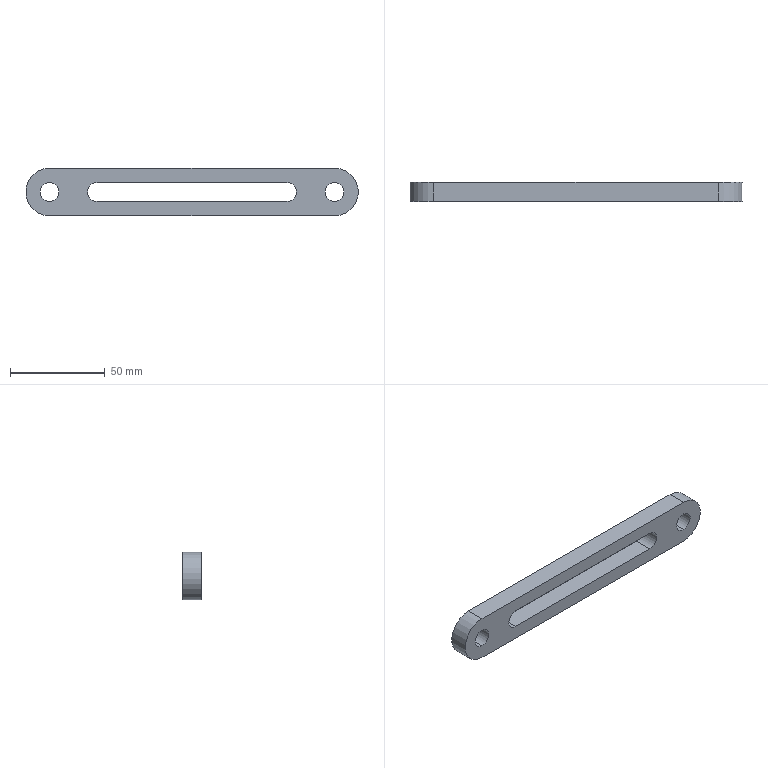Part | SolidWorks | features Extrusion 1, ICE 1 | 1 solid | 14 faces | box 175 x 10 x 25 mm | volume 30053 mm3 | cylinder 8 | plane 6 | commonest cylinder face diameters 10 x6 25 x2
STEP:
#1=CARTESIAN_POINT('',(150.,5.,-5.));
#2=VERTEX_POINT('',#1);
#3=CARTESIAN_POINT('',(150.,5.,5.));
#4=VERTEX_POINT('',#3);
#5=CARTESIAN_POINT('',(150.,5.,0.));
#6=DIRECTION('',(0.,1.,0.));
#7=DIRECTION('',(0.,0.,1.));
#8=AXIS2_PLACEMENT_3D('',#5,#6,#7);
#9=CIRCLE('',#8,5.);
#10=EDGE_CURVE('',#2,#4,#9,.T.);
#11=ORIENTED_EDGE('',*,*,#10,.T.);
#12=CARTESIAN_POINT('',(150.,-5.,5.));
#13=VERTEX_POINT('',#12);
#14=CARTESIAN_POINT('',(150.,5.,5.));
#15=DIRECTION('',(0.,-1.,0.));
#16=VECTOR('',#15,1000.);
#17=LINE('',#14,#16);
#18=EDGE_CURVE('',#4,#13,#17,.T.);
#19=ORIENTED_EDGE('',*,*,#18,.T.);
#20=CARTESIAN_POINT('',(150.,-5.,-5.));
#21=VERTEX_POINT('',#20);
#22=CARTESIAN_POINT('',(150.,-5.,0.));
#23=DIRECTION('',(0.,1.,0.));
#24=DIRECTION('',(0.,0.,1.));
#25=AXIS2_PLACEMENT_3D('',#22,#23,#24);
#26=CIRCLE('',#25,5.);
#27=EDGE_CURVE('',#21,#13,#26,.T.);
#28=ORIENTED_EDGE('',*,*,#27,.F.);
#29=CARTESIAN_POINT('',(150.,5.,-5.));
#30=DIRECTION('',(0.,-1.,0.));
#31=VECTOR('',#30,1000.);
#32=LINE('',#29,#31);
#33=EDGE_CURVE('',#2,#21,#32,.T.);
#34=ORIENTED_EDGE('',*,*,#33,.F.);
#35=EDGE_LOOP('',(#11,#19,#28,#34));
#36=FACE_OUTER_BOUND('',#35,.T.);
#37=CARTESIAN_POINT('',(150.,5.,0.));
#38=DIRECTION('',(0.,-1.,0.));
#39=DIRECTION('',(0.,0.,-1.));
#40=AXIS2_PLACEMENT_3D('',#37,#38,#39);
#41=CYLINDRICAL_SURFACE('',#40,5.);
#42=ADVANCED_FACE('',(#36),#41,.F.);
#43=CARTESIAN_POINT('',(0.,5.,-5.));
#44=VERTEX_POINT('',#43);
#45=CARTESIAN_POINT('',(0.,5.,5.));
#46=VERTEX_POINT('',#45);
#47=CARTESIAN_POINT('',(0.,5.,0.));
#48=DIRECTION('',(0.,1.,0.));
#49=DIRECTION('',(0.,0.,1.));
#50=AXIS2_PLACEMENT_3D('',#47,#48,#49);
#51=CIRCLE('',#50,5.);
#52=EDGE_CURVE('',#44,#46,#51,.T.);
#53=ORIENTED_EDGE('',*,*,#52,.T.);
#54=CARTESIAN_POINT('',(0.,-5.,5.));
#55=VERTEX_POINT('',#54);
#56=CARTESIAN_POINT('',(0.,5.,5.));
#57=DIRECTION('',(0.,-1.,0.));
#58=VECTOR('',#57,1000.);
#59=LINE('',#56,#58);
#60=EDGE_CURVE('',#46,#55,#59,.T.);
#61=ORIENTED_EDGE('',*,*,#60,.T.);
#62=CARTESIAN_POINT('',(0.,-5.,-5.));
#63=VERTEX_POINT('',#62);
#64=CARTESIAN_POINT('',(0.,-5.,0.));
#65=DIRECTION('',(0.,1.,0.));
#66=DIRECTION('',(0.,0.,1.));
#67=AXIS2_PLACEMENT_3D('',#64,#65,#66);
#68=CIRCLE('',#67,5.);
#69=EDGE_CURVE('',#63,#55,#68,.T.);
#70=ORIENTED_EDGE('',*,*,#69,.F.);
#71=CARTESIAN_POINT('',(0.,5.,-5.));
#72=DIRECTION('',(0.,-1.,0.));
#73=VECTOR('',#72,1000.);
#74=LINE('',#71,#73);
#75=EDGE_CURVE('',#44,#63,#74,.T.);
#76=ORIENTED_EDGE('',*,*,#75,.F.);
#77=EDGE_LOOP('',(#53,#61,#70,#76));
#78=FACE_OUTER_BOUND('',#77,.T.);
#79=CARTESIAN_POINT('',(0.,5.,0.));
#80=DIRECTION('',(0.,-1.,0.));
#81=DIRECTION('',(0.,0.,-1.));
#82=AXIS2_PLACEMENT_3D('',#79,#80,#81);
#83=CYLINDRICAL_SURFACE('',#82,5.);
#84=ADVANCED_FACE('',(#78),#83,.F.);
#85=CARTESIAN_POINT('',(25.,5.,-5.));
#86=VERTEX_POINT('',#85);
#87=CARTESIAN_POINT('',(25.,5.,5.));
#88=VERTEX_POINT('',#87);
#89=CARTESIAN_POINT('',(25.,5.,0.));
#90=DIRECTION('',(0.,1.,0.));
#91=DIRECTION('',(0.,0.,1.));
#92=AXIS2_PLACEMENT_3D('',#89,#90,#91);
#93=CIRCLE('',#92,5.);
#94=EDGE_CURVE('',#86,#88,#93,.T.);
#95=ORIENTED_EDGE('',*,*,#94,.F.);
#96=CARTESIAN_POINT('',(125.,5.,-5.));
#97=VERTEX_POINT('',#96);
#98=CARTESIAN_POINT('',(25.,5.,-5.));
#99=DIRECTION('',(-1.,0.,0.));
#100=VECTOR('',#99,1000.);
#101=LINE('',#98,#100);
#102=EDGE_CURVE('',#97,#86,#101,.T.);
#103=ORIENTED_EDGE('',*,*,#102,.F.);
#104=CARTESIAN_POINT('',(125.,5.,5.));
#105=VERTEX_POINT('',#104);
#106=CARTESIAN_POINT('',(125.,5.,0.));
#107=DIRECTION('',(0.,1.,0.));
#108=DIRECTION('',(0.,0.,1.));
#109=AXIS2_PLACEMENT_3D('',#106,#107,#108);
#110=CIRCLE('',#109,5.);
#111=EDGE_CURVE('',#105,#97,#110,.T.);
#112=ORIENTED_EDGE('',*,*,#111,.F.);
#113=CARTESIAN_POINT('',(25.,5.,5.));
#114=DIRECTION('',(1.,0.,0.));
#115=VECTOR('',#114,1000.);
#116=LINE('',#113,#115);
#117=EDGE_CURVE('',#88,#105,#116,.T.);
#118=ORIENTED_EDGE('',*,*,#117,.F.);
#119=EDGE_LOOP('',(#95,#103,#112,#118));
#120=FACE_BOUND('',#119,.T.);
#121=ORIENTED_EDGE('',*,*,#52,.F.);
#122=CARTESIAN_POINT('',(0.,5.,0.));
#123=DIRECTION('',(0.,1.,0.));
#124=DIRECTION('',(0.,0.,1.));
#125=AXIS2_PLACEMENT_3D('',#122,#123,#124);
#126=CIRCLE('',#125,5.);
#127=EDGE_CURVE('',#46,#44,#126,.T.);
#128=ORIENTED_EDGE('',*,*,#127,.F.);
#129=EDGE_LOOP('',(#121,#128));
#130=FACE_BOUND('',#129,.T.);
#131=CARTESIAN_POINT('',(0.,5.,-12.5));
#132=VERTEX_POINT('',#131);
#133=CARTESIAN_POINT('',(0.,5.,12.5));
#134=VERTEX_POINT('',#133);
#135=CARTESIAN_POINT('',(0.,5.,0.));
#136=DIRECTION('',(0.,1.,0.));
#137=DIRECTION('',(0.,0.,1.));
#138=AXIS2_PLACEMENT_3D('',#135,#136,#137);
#139=CIRCLE('',#138,12.5);
#140=EDGE_CURVE('',#132,#134,#139,.T.);
#141=ORIENTED_EDGE('',*,*,#140,.T.);
#142=CARTESIAN_POINT('',(150.,5.,12.5));
#143=VERTEX_POINT('',#142);
#144=CARTESIAN_POINT('',(0.,5.,12.5));
#145=DIRECTION('',(1.,0.,0.));
#146=VECTOR('',#145,1000.);
#147=LINE('',#144,#146);
#148=EDGE_CURVE('',#134,#143,#147,.T.);
#149=ORIENTED_EDGE('',*,*,#148,.T.);
#150=CARTESIAN_POINT('',(150.,5.,-12.5));
#151=VERTEX_POINT('',#150);
#152=CARTESIAN_POINT('',(150.,5.,0.));
#153=DIRECTION('',(0.,1.,0.));
#154=DIRECTION('',(0.,0.,1.));
#155=AXIS2_PLACEMENT_3D('',#152,#153,#154);
#156=CIRCLE('',#155,12.5);
#157=EDGE_CURVE('',#143,#151,#156,.T.);
#158=ORIENTED_EDGE('',*,*,#157,.T.);
#159=CARTESIAN_POINT('',(0.,5.,-12.5));
#160=DIRECTION('',(-1.,0.,0.));
#161=VECTOR('',#160,1000.);
#162=LINE('',#159,#161);
#163=EDGE_CURVE('',#151,#132,#162,.T.);
#164=ORIENTED_EDGE('',*,*,#163,.T.);
#165=EDGE_LOOP('',(#141,#149,#158,#164));
#166=FACE_OUTER_BOUND('',#165,.T.);
#167=ORIENTED_EDGE('',*,*,#10,.F.);
#168=CARTESIAN_POINT('',(150.,5.,0.));
#169=DIRECTION('',(0.,1.,0.));
#170=DIRECTION('',(0.,0.,1.));
#171=AXIS2_PLACEMENT_3D('',#168,#169,#170);
#172=CIRCLE('',#171,5.);
#173=EDGE_CURVE('',#4,#2,#172,.T.);
#174=ORIENTED_EDGE('',*,*,#173,.F.);
#175=EDGE_LOOP('',(#167,#174));
#176=FACE_BOUND('',#175,.T.);
#177=CARTESIAN_POINT('',(0.,5.,0.));
#178=DIRECTION('',(0.,1.,0.));
#179=DIRECTION('',(0.,0.,1.));
#180=AXIS2_PLACEMENT_3D('',#177,#178,#179);
#181=PLANE('',#180);
#182=ADVANCED_FACE('',(#120,#130,#166,#176),#181,.T.);
#183=CARTESIAN_POINT('',(125.,-5.,-5.));
#184=VERTEX_POINT('',#183);
#185=CARTESIAN_POINT('',(25.,-5.,-5.));
#186=VERTEX_POINT('',#185);
#187=CARTESIAN_POINT('',(25.,-5.,-5.));
#188=DIRECTION('',(-1.,0.,0.));
#189=VECTOR('',#188,1000.);
#190=LINE('',#187,#189);
#191=EDGE_CURVE('',#184,#186,#190,.T.);
#192=ORIENTED_EDGE('',*,*,#191,.T.);
#193=CARTESIAN_POINT('',(25.,-5.,5.));
#194=VERTEX_POINT('',#193);
#195=CARTESIAN_POINT('',(25.,-5.,0.));
#196=DIRECTION('',(0.,1.,0.));
#197=DIRECTION('',(0.,0.,1.));
#198=AXIS2_PLACEMENT_3D('',#195,#196,#197);
#199=CIRCLE('',#198,5.);
#200=EDGE_CURVE('',#186,#194,#199,.T.);
#201=ORIENTED_EDGE('',*,*,#200,.T.);
#202=CARTESIAN_POINT('',(125.,-5.,5.));
#203=VERTEX_POINT('',#202);
#204=CARTESIAN_POINT('',(25.,-5.,5.));
#205=DIRECTION('',(1.,0.,0.));
#206=VECTOR('',#205,1000.);
#207=LINE('',#204,#206);
#208=EDGE_CURVE('',#194,#203,#207,.T.);
#209=ORIENTED_EDGE('',*,*,#208,.T.);
#210=CARTESIAN_POINT('',(125.,-5.,0.));
#211=DIRECTION('',(0.,1.,0.));
#212=DIRECTION('',(0.,0.,1.));
#213=AXIS2_PLACEMENT_3D('',#210,#211,#212);
#214=CIRCLE('',#213,5.);
#215=EDGE_CURVE('',#203,#184,#214,.T.);
#216=ORIENTED_EDGE('',*,*,#215,.T.);
#217=EDGE_LOOP('',(#192,#201,#209,#216));
#218=FACE_BOUND('',#217,.T.);
#219=CARTESIAN_POINT('',(0.,-5.,-12.5));
#220=VERTEX_POINT('',#219);
#221=CARTESIAN_POINT('',(0.,-5.,12.5));
#222=VERTEX_POINT('',#221);
#223=CARTESIAN_POINT('',(0.,-5.,0.));
#224=DIRECTION('',(0.,1.,0.));
#225=DIRECTION('',(0.,0.,1.));
#226=AXIS2_PLACEMENT_3D('',#223,#224,#225);
#227=CIRCLE('',#226,12.5);
#228=EDGE_CURVE('',#220,#222,#227,.T.);
#229=ORIENTED_EDGE('',*,*,#228,.F.);
#230=CARTESIAN_POINT('',(150.,-5.,-12.5));
#231=VERTEX_POINT('',#230);
#232=CARTESIAN_POINT('',(0.,-5.,-12.5));
#233=DIRECTION('',(-1.,0.,0.));
#234=VECTOR('',#233,1000.);
#235=LINE('',#232,#234);
#236=EDGE_CURVE('',#231,#220,#235,.T.);
#237=ORIENTED_EDGE('',*,*,#236,.F.);
#238=CARTESIAN_POINT('',(150.,-5.,12.5));
#239=VERTEX_POINT('',#238);
#240=CARTESIAN_POINT('',(150.,-5.,0.));
#241=DIRECTION('',(0.,1.,0.));
#242=DIRECTION('',(0.,0.,1.));
#243=AXIS2_PLACEMENT_3D('',#240,#241,#242);
#244=CIRCLE('',#243,12.5);
#245=EDGE_CURVE('',#239,#231,#244,.T.);
#246=ORIENTED_EDGE('',*,*,#245,.F.);
#247=CARTESIAN_POINT('',(0.,-5.,12.5));
#248=DIRECTION('',(1.,0.,0.));
#249=VECTOR('',#248,1000.);
#250=LINE('',#247,#249);
#251=EDGE_CURVE('',#222,#239,#250,.T.);
#252=ORIENTED_EDGE('',*,*,#251,.F.);
#253=EDGE_LOOP('',(#229,#237,#246,#252));
#254=FACE_OUTER_BOUND('',#253,.T.);
#255=ORIENTED_EDGE('',*,*,#69,.T.);
#256=CARTESIAN_POINT('',(0.,-5.,0.));
#257=DIRECTION('',(0.,1.,0.));
#258=DIRECTION('',(0.,0.,1.));
#259=AXIS2_PLACEMENT_3D('',#256,#257,#258);
#260=CIRCLE('',#259,5.);
#261=EDGE_CURVE('',#55,#63,#260,.T.);
#262=ORIENTED_EDGE('',*,*,#261,.T.);
#263=EDGE_LOOP('',(#255,#262));
#264=FACE_BOUND('',#263,.T.);
#265=ORIENTED_EDGE('',*,*,#27,.T.);
#266=CARTESIAN_POINT('',(150.,-5.,0.));
#267=DIRECTION('',(0.,1.,0.));
#268=DIRECTION('',(0.,0.,1.));
#269=AXIS2_PLACEMENT_3D('',#266,#267,#268);
#270=CIRCLE('',#269,5.);
#271=EDGE_CURVE('',#13,#21,#270,.T.);
#272=ORIENTED_EDGE('',*,*,#271,.T.);
#273=EDGE_LOOP('',(#265,#272));
#274=FACE_BOUND('',#273,.T.);
#275=CARTESIAN_POINT('',(0.,-5.,0.));
#276=DIRECTION('',(0.,1.,0.));
#277=DIRECTION('',(0.,0.,1.));
#278=AXIS2_PLACEMENT_3D('',#275,#276,#277);
#279=PLANE('',#278);
#280=ADVANCED_FACE('',(#218,#254,#264,#274),#279,.F.);
#281=ORIENTED_EDGE('',*,*,#228,.T.);
#282=CARTESIAN_POINT('',(0.,5.,12.5));
#283=DIRECTION('',(0.,-1.,0.));
#284=VECTOR('',#283,1000.);
#285=LINE('',#282,#284);
#286=EDGE_CURVE('',#134,#222,#285,.T.);
#287=ORIENTED_EDGE('',*,*,#286,.F.);
#288=ORIENTED_EDGE('',*,*,#140,.F.);
#289=CARTESIAN_POINT('',(0.,5.,-12.5));
#290=DIRECTION('',(0.,-1.,0.));
#291=VECTOR('',#290,1000.);
#292=LINE('',#289,#291);
#293=EDGE_CURVE('',#132,#220,#292,.T.);
#294=ORIENTED_EDGE('',*,*,#293,.T.);
#295=EDGE_LOOP('',(#281,#287,#288,#294));
#296=FACE_OUTER_BOUND('',#295,.T.);
#297=CARTESIAN_POINT('',(0.,5.,0.));
#298=DIRECTION('',(0.,-1.,0.));
#299=DIRECTION('',(0.,0.,-1.));
#300=AXIS2_PLACEMENT_3D('',#297,#298,#299);
#301=CYLINDRICAL_SURFACE('',#300,12.5);
#302=ADVANCED_FACE('',(#296),#301,.T.);
#303=ORIENTED_EDGE('',*,*,#251,.T.);
#304=CARTESIAN_POINT('',(150.,5.,12.5));
#305=DIRECTION('',(0.,-1.,0.));
#306=VECTOR('',#305,1000.);
#307=LINE('',#304,#306);
#308=EDGE_CURVE('',#143,#239,#307,.T.);
#309=ORIENTED_EDGE('',*,*,#308,.F.);
#310=ORIENTED_EDGE('',*,*,#148,.F.);
#311=ORIENTED_EDGE('',*,*,#286,.T.);
#312=EDGE_LOOP('',(#303,#309,#310,#311));
#313=FACE_OUTER_BOUND('',#312,.T.);
#314=CARTESIAN_POINT('',(0.,5.,12.5));
#315=DIRECTION('',(0.,0.,-1.));
#316=DIRECTION('',(-1.,0.,0.));
#317=AXIS2_PLACEMENT_3D('',#314,#315,#316);
#318=PLANE('',#317);
#319=ADVANCED_FACE('',(#313),#318,.F.);
#320=ORIENTED_EDGE('',*,*,#245,.T.);
#321=CARTESIAN_POINT('',(150.,5.,-12.5));
#322=DIRECTION('',(0.,-1.,0.));
#323=VECTOR('',#322,1000.);
#324=LINE('',#321,#323);
#325=EDGE_CURVE('',#151,#231,#324,.T.);
#326=ORIENTED_EDGE('',*,*,#325,.F.);
#327=ORIENTED_EDGE('',*,*,#157,.F.);
#328=ORIENTED_EDGE('',*,*,#308,.T.);
#329=EDGE_LOOP('',(#320,#326,#327,#328));
#330=FACE_OUTER_BOUND('',#329,.T.);
#331=CARTESIAN_POINT('',(150.,5.,0.));
#332=DIRECTION('',(0.,-1.,0.));
#333=DIRECTION('',(0.,0.,-1.));
#334=AXIS2_PLACEMENT_3D('',#331,#332,#333);
#335=CYLINDRICAL_SURFACE('',#334,12.5);
#336=ADVANCED_FACE('',(#330),#335,.T.);
#337=ORIENTED_EDGE('',*,*,#236,.T.);
#338=ORIENTED_EDGE('',*,*,#293,.F.);
#339=ORIENTED_EDGE('',*,*,#163,.F.);
#340=ORIENTED_EDGE('',*,*,#325,.T.);
#341=EDGE_LOOP('',(#337,#338,#339,#340));
#342=FACE_OUTER_BOUND('',#341,.T.);
#343=CARTESIAN_POINT('',(0.,5.,-12.5));
#344=DIRECTION('',(0.,0.,1.));
#345=DIRECTION('',(1.,0.,0.));
#346=AXIS2_PLACEMENT_3D('',#343,#344,#345);
#347=PLANE('',#346);
#348=ADVANCED_FACE('',(#342),#347,.F.);
#349=ORIENTED_EDGE('',*,*,#60,.F.);
#350=ORIENTED_EDGE('',*,*,#127,.T.);
#351=ORIENTED_EDGE('',*,*,#75,.T.);
#352=ORIENTED_EDGE('',*,*,#261,.F.);
#353=EDGE_LOOP('',(#349,#350,#351,#352));
#354=FACE_OUTER_BOUND('',#353,.T.);
#355=CARTESIAN_POINT('',(0.,5.,0.));
#356=DIRECTION('',(0.,-1.,0.));
#357=DIRECTION('',(0.,0.,-1.));
#358=AXIS2_PLACEMENT_3D('',#355,#356,#357);
#359=CYLINDRICAL_SURFACE('',#358,5.);
#360=ADVANCED_FACE('',(#354),#359,.F.);
#361=ORIENTED_EDGE('',*,*,#18,.F.);
#362=ORIENTED_EDGE('',*,*,#173,.T.);
#363=ORIENTED_EDGE('',*,*,#33,.T.);
#364=ORIENTED_EDGE('',*,*,#271,.F.);
#365=EDGE_LOOP('',(#361,#362,#363,#364));
#366=FACE_OUTER_BOUND('',#365,.T.);
#367=CARTESIAN_POINT('',(150.,5.,0.));
#368=DIRECTION('',(0.,-1.,0.));
#369=DIRECTION('',(0.,0.,-1.));
#370=AXIS2_PLACEMENT_3D('',#367,#368,#369);
#371=CYLINDRICAL_SURFACE('',#370,5.);
#372=ADVANCED_FACE('',(#366),#371,.F.);
#373=ORIENTED_EDGE('',*,*,#94,.T.);
#374=CARTESIAN_POINT('',(25.,-5.,5.));
#375=DIRECTION('',(0.,1.,0.));
#376=VECTOR('',#375,1000.);
#377=LINE('',#374,#376);
#378=EDGE_CURVE('',#194,#88,#377,.T.);
#379=ORIENTED_EDGE('',*,*,#378,.F.);
#380=ORIENTED_EDGE('',*,*,#200,.F.);
#381=CARTESIAN_POINT('',(25.,-5.,-5.));
#382=DIRECTION('',(0.,1.,0.));
#383=VECTOR('',#382,1000.);
#384=LINE('',#381,#383);
#385=EDGE_CURVE('',#186,#86,#384,.T.);
#386=ORIENTED_EDGE('',*,*,#385,.T.);
#387=EDGE_LOOP('',(#373,#379,#380,#386));
#388=FACE_OUTER_BOUND('',#387,.T.);
#389=CARTESIAN_POINT('',(25.,-5.,0.));
#390=DIRECTION('',(0.,1.,0.));
#391=DIRECTION('',(0.,0.,1.));
#392=AXIS2_PLACEMENT_3D('',#389,#390,#391);
#393=CYLINDRICAL_SURFACE('',#392,5.);
#394=ADVANCED_FACE('',(#388),#393,.F.);
#395=ORIENTED_EDGE('',*,*,#102,.T.);
#396=ORIENTED_EDGE('',*,*,#385,.F.);
#397=ORIENTED_EDGE('',*,*,#191,.F.);
#398=CARTESIAN_POINT('',(125.,-5.,-5.));
#399=DIRECTION('',(0.,1.,0.));
#400=VECTOR('',#399,1000.);
#401=LINE('',#398,#400);
#402=EDGE_CURVE('',#184,#97,#401,.T.);
#403=ORIENTED_EDGE('',*,*,#402,.T.);
#404=EDGE_LOOP('',(#395,#396,#397,#403));
#405=FACE_OUTER_BOUND('',#404,.T.);
#406=CARTESIAN_POINT('',(25.,-5.,-5.));
#407=DIRECTION('',(0.,0.,-1.));
#408=DIRECTION('',(-1.,0.,0.));
#409=AXIS2_PLACEMENT_3D('',#406,#407,#408);
#410=PLANE('',#409);
#411=ADVANCED_FACE('',(#405),#410,.F.);
#412=ORIENTED_EDGE('',*,*,#111,.T.);
#413=ORIENTED_EDGE('',*,*,#402,.F.);
#414=ORIENTED_EDGE('',*,*,#215,.F.);
#415=CARTESIAN_POINT('',(125.,-5.,5.));
#416=DIRECTION('',(0.,1.,0.));
#417=VECTOR('',#416,1000.);
#418=LINE('',#415,#417);
#419=EDGE_CURVE('',#203,#105,#418,.T.);
#420=ORIENTED_EDGE('',*,*,#419,.T.);
#421=EDGE_LOOP('',(#412,#413,#414,#420));
#422=FACE_OUTER_BOUND('',#421,.T.);
#423=CARTESIAN_POINT('',(125.,-5.,0.));
#424=DIRECTION('',(0.,1.,0.));
#425=DIRECTION('',(0.,0.,1.));
#426=AXIS2_PLACEMENT_3D('',#423,#424,#425);
#427=CYLINDRICAL_SURFACE('',#426,5.);
#428=ADVANCED_FACE('',(#422),#427,.F.);
#429=ORIENTED_EDGE('',*,*,#117,.T.);
#430=ORIENTED_EDGE('',*,*,#419,.F.);
#431=ORIENTED_EDGE('',*,*,#208,.F.);
#432=ORIENTED_EDGE('',*,*,#378,.T.);
#433=EDGE_LOOP('',(#429,#430,#431,#432));
#434=FACE_OUTER_BOUND('',#433,.T.);
#435=CARTESIAN_POINT('',(25.,-5.,5.));
#436=DIRECTION('',(0.,0.,1.));
#437=DIRECTION('',(1.,0.,0.));
#438=AXIS2_PLACEMENT_3D('',#435,#436,#437);
#439=PLANE('',#438);
#440=ADVANCED_FACE('',(#434),#439,.F.);
#441=CLOSED_SHELL('',(#42,#84,#182,#280,#302,#319,#336,#348,#360,#372,#394,#411,#428,#440));
#442=MANIFOLD_SOLID_BREP('',#441);
#443=CARTESIAN_POINT('',(0.,0.,0.));
#444=DIRECTION('',(0.,0.,1.));
#445=DIRECTION('',(1.,0.,0.));
#446=AXIS2_PLACEMENT_3D('',#443,#444,#445);
#447=(LENGTH_UNIT()NAMED_UNIT(*)SI_UNIT(.MILLI.,.METRE.));
#448=UNCERTAINTY_MEASURE_WITH_UNIT(LENGTH_MEASURE(0.00001),#447,'','');
#449=(NAMED_UNIT(*)PLANE_ANGLE_UNIT()SI_UNIT($,.RADIAN.));
#450=(NAMED_UNIT(*)SI_UNIT($,.STERADIAN.)SOLID_ANGLE_UNIT());
#451=(GEOMETRIC_REPRESENTATION_CONTEXT(3)GLOBAL_UNCERTAINTY_ASSIGNED_CONTEXT((#448))GLOBAL_UNIT_ASSIGNED_CONTEXT((#447,#449,#450))REPRESENTATION_CONTEXT('',''));
#452=ADVANCED_BREP_SHAPE_REPRESENTATION('',(#442,#446),#451);